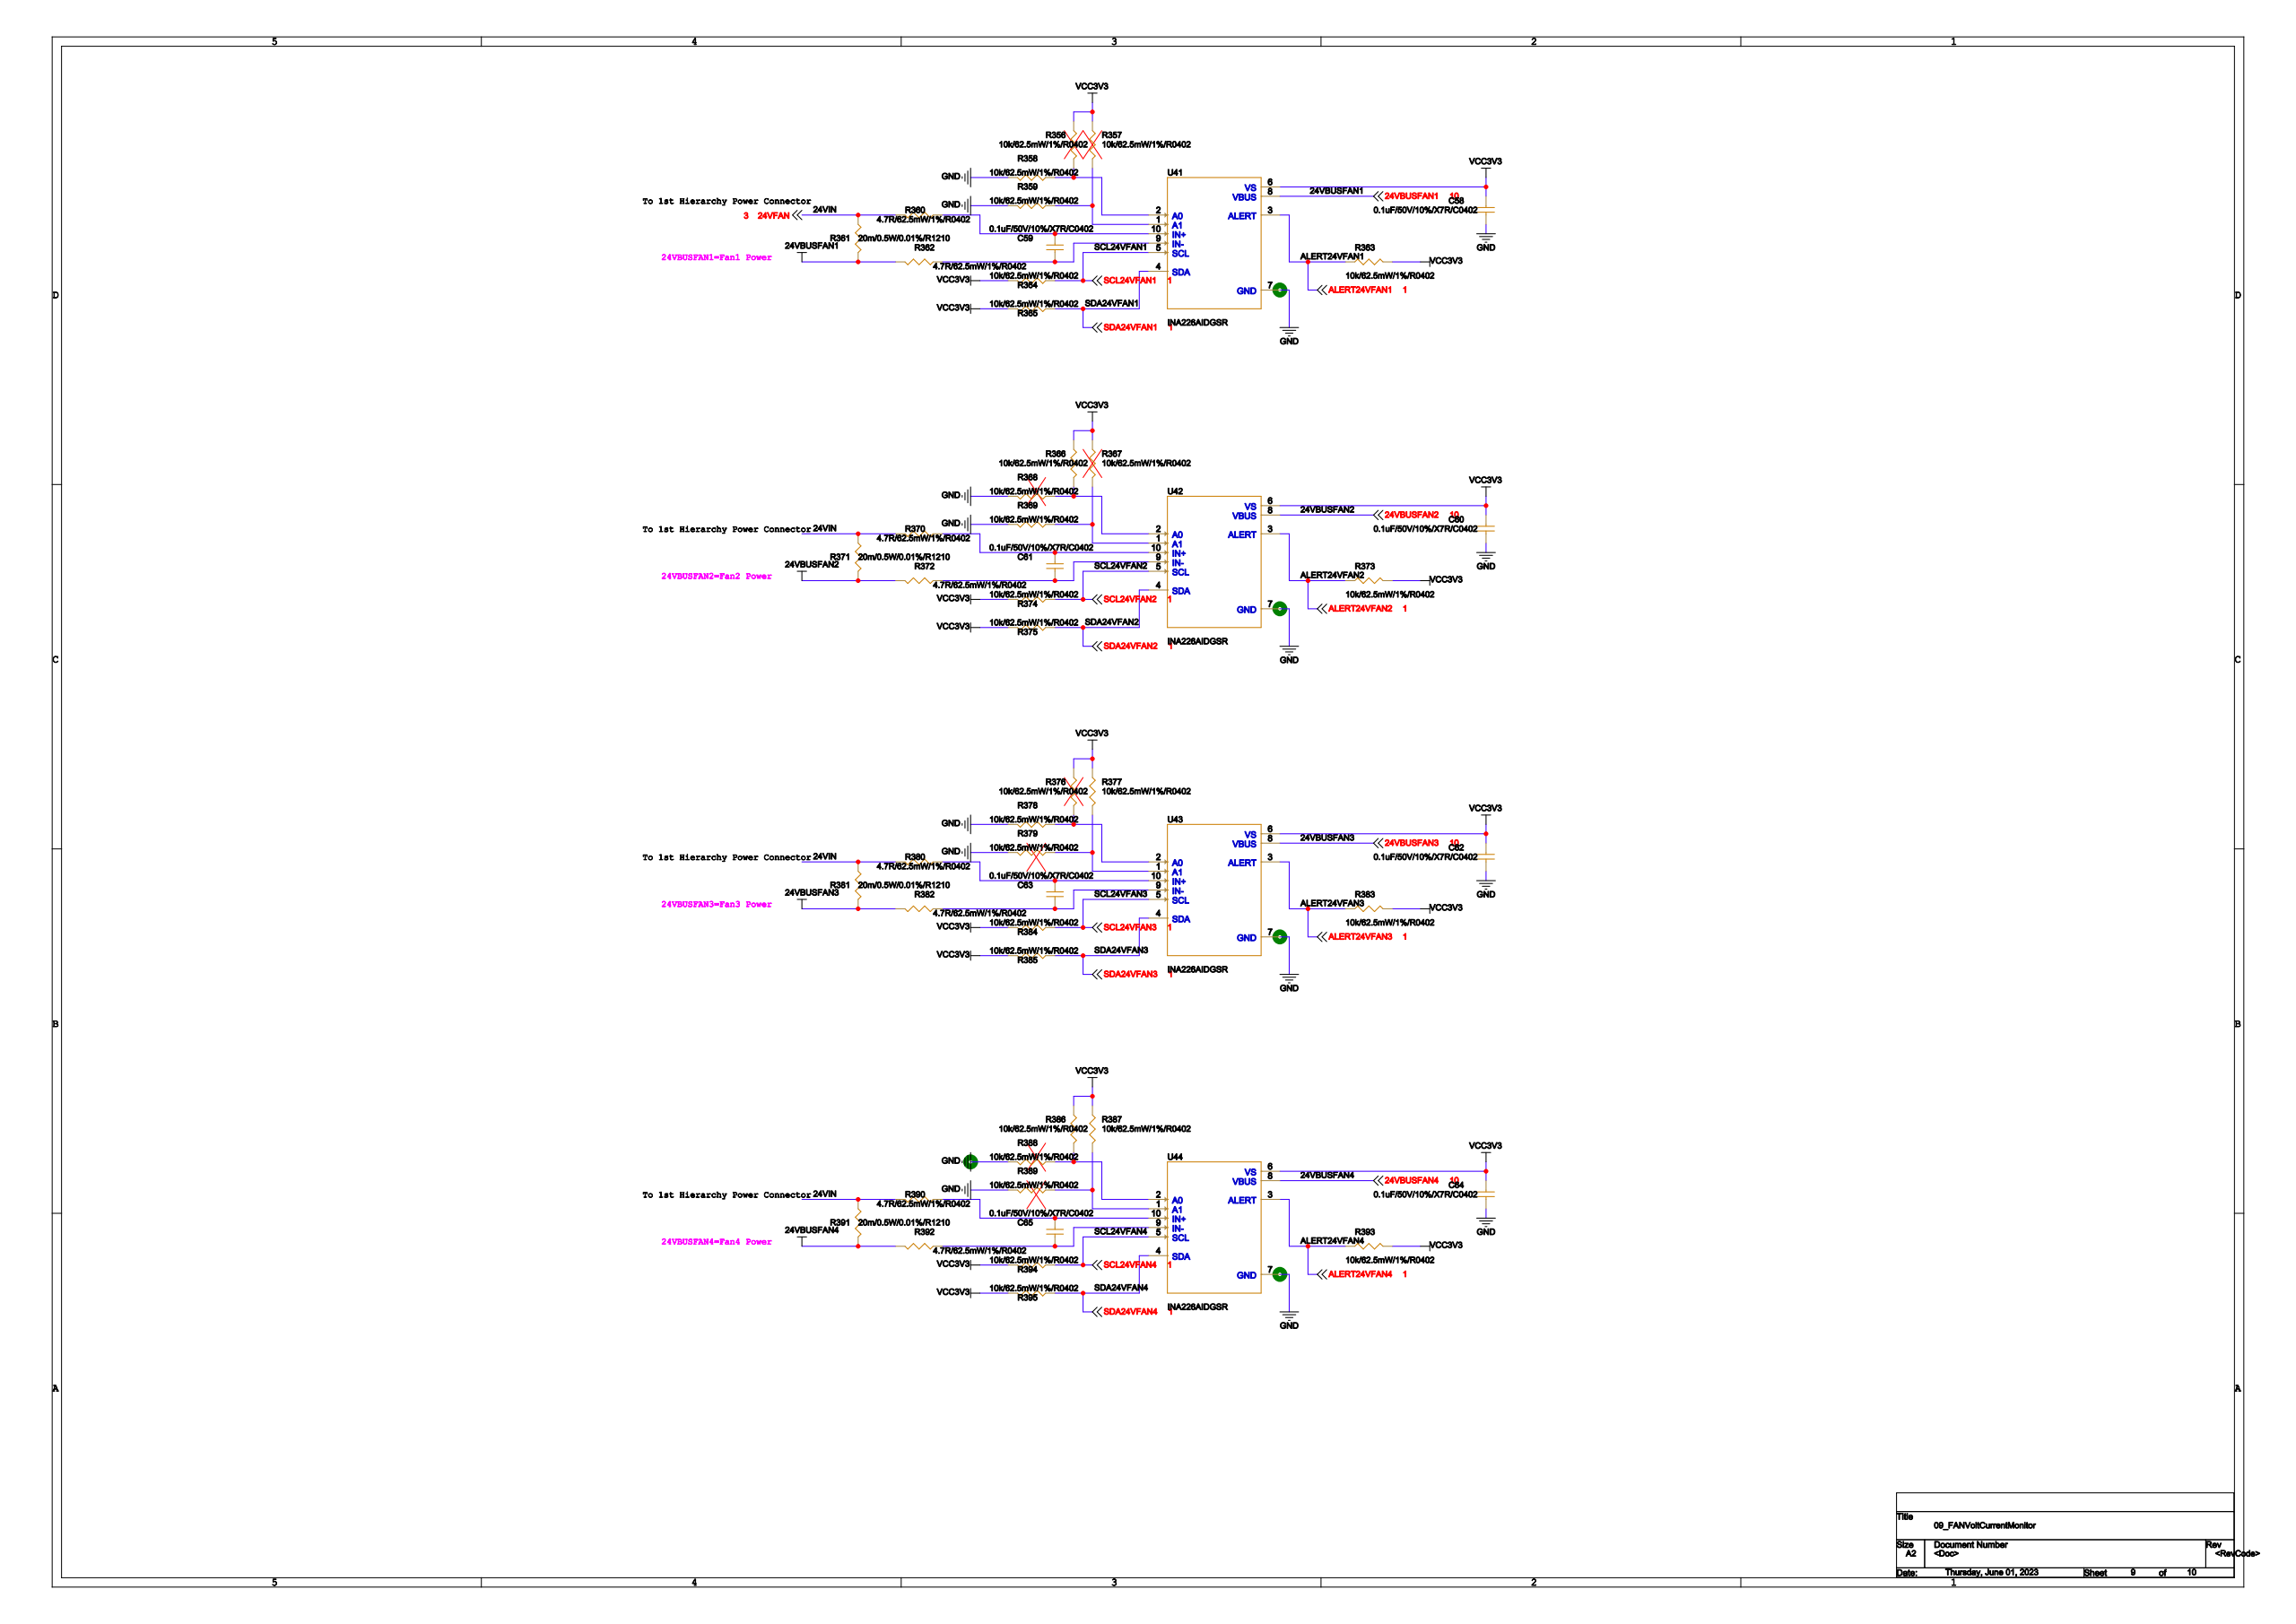Circuit board | Cadence Allegro | 480 parts | 625 nets | one sheet of the schematic
Parts on this sheet (reference | value | footprint):
C58 | 0.1uF/50V/10%/X7R/C0402 | 0402
C59 | 0.1uF/50V/10%/X7R/C0402 | 0402
C60 | 0.1uF/50V/10%/X7R/C0402 | 0402
C61 | 0.1uF/50V/10%/X7R/C0402 | 0402
C62 | 0.1uF/50V/10%/X7R/C0402 | 0402
C63 | 0.1uF/50V/10%/X7R/C0402 | 0402
C64 | 0.1uF/50V/10%/X7R/C0402 | 0402
C65 | 0.1uF/50V/10%/X7R/C0402 | 0402
R356 | 10k/62.5mW/1%/R0402 | 0402
R357 | 10k/62.5mW/1%/R0402 | 0402
R358 | 10k/62.5mW/1%/R0402 | 0402
R359 | 10k/62.5mW/1%/R0402 | 0402
R360 | 4.7R/62.5mW/1%/R0402 | 0402
R361 | 20m/0.5W/0.01%/R1210 | 1210
R362 | 4.7R/62.5mW/1%/R0402 | 0402
R363 | 10k/62.5mW/1%/R0402 | 0402
R364 | 10k/62.5mW/1%/R0402 | 0402
R365 | 10k/62.5mW/1%/R0402 | 0402
R366 | 10k/62.5mW/1%/R0402 | 0402
R367 | 10k/62.5mW/1%/R0402 | 0402
R368 | 10k/62.5mW/1%/R0402 | 0402
R369 | 10k/62.5mW/1%/R0402 | 0402
R370 | 4.7R/62.5mW/1%/R0402 | 0402
R371 | 20m/0.5W/0.01%/R1210 | 1210
R372 | 4.7R/62.5mW/1%/R0402 | 0402
R373 | 10k/62.5mW/1%/R0402 | 0402
R374 | 10k/62.5mW/1%/R0402 | 0402
R375 | 10k/62.5mW/1%/R0402 | 0402
R376 | 10k/62.5mW/1%/R0402 | 0402
R377 | 10k/62.5mW/1%/R0402 | 0402
R378 | 10k/62.5mW/1%/R0402 | 0402
R379 | 10k/62.5mW/1%/R0402 | 0402
R380 | 4.7R/62.5mW/1%/R0402 | 0402
R381 | 20m/0.5W/0.01%/R1210 | 1210
R382 | 4.7R/62.5mW/1%/R0402 | 0402
R383 | 10k/62.5mW/1%/R0402 | 0402
R384 | 10k/62.5mW/1%/R0402 | 0402
R385 | 10k/62.5mW/1%/R0402 | 0402
R386 | 10k/62.5mW/1%/R0402 | 0402
R387 | 10k/62.5mW/1%/R0402 | 0402
R388 | 10k/62.5mW/1%/R0402 | 0402
R389 | 10k/62.5mW/1%/R0402 | 0402
R390 | 4.7R/62.5mW/1%/R0402 | 0402
R391 | 20m/0.5W/0.01%/R1210 | 1210
R392 | 4.7R/62.5mW/1%/R0402 | 0402
R393 | 10k/62.5mW/1%/R0402 | 0402
R394 | 10k/62.5mW/1%/R0402 | 0402
R395 | 10k/62.5mW/1%/R0402 | 0402
U41 | INA226AIDGSR | SOP50P490X110-10N
U42 | INA226AIDGSR | SOP50P490X110-10N
U43 | INA226AIDGSR | SOP50P490X110-10N
U44 | INA226AIDGSR | SOP50P490X110-10N
Nets of these parts (net: part-pin ...):
AGND: C58-2 C60-2 C62-2 C64-2 R358-2 R359-2 R368-2 R369-2 R378-2 R379-2 R388-2 R389-2 U41-7 U42-7 U43-7 U44-7
BANK13_L5_N: R364-1 U41-5
ALERT24VFAN4: R393-1 U44-3
BANK13_L6_P: R365-1 U41-4
BANK13_L12_N: R395-1 U44-4
ALERT24VFAN1: R363-1 U41-3
BANK13_L4_N: R394-1 U44-5
BANK13_L5_P: R374-1 U42-5
ALERT24VFAN3: R383-1 U43-3
BANK13_L21_P: R375-1 U42-4
BANK13_L14_P: R385-1 U43-4
ALERT24VFAN2: R373-1 U42-3
BANK13_L17_N: R384-1 U43-5
3.3V: C58-1 C60-1 C62-1 C64-1 R356-1 R357-1 R363-2 R364-2 R365-2 R366-1 R367-1 R373-2 R374-2 R375-2 R376-1 R377-1 R383-2 R384-2 R385-2 R386-1 R387-1 R393-2 R394-2 R395-2 U41-6 U42-6 U43-6 U44-6
24VBUSFAN1: R361-2 R362-2 U41-8
24VBUSFAN4: R391-2 R392-2 U44-8
24VBUSFAN2: R371-2 R372-2 U42-8
24VBUSFAN3: R381-2 R382-2 U43-8
24VFAN: R360-2 R361-1 R370-2 R371-1 R380-2 R381-1 R390-2 R391-1
N23136700: C59-1 R360-1 U41-10
N23136726: C59-2 R362-1 U41-9
N23189446: C61-1 R370-1 U42-10
N23189612: C61-2 R372-1 U42-9
N23190079: C63-1 R380-1 U43-10
N23190245: C63-2 R382-1 U43-9
N23190745: C65-1 R390-1 U44-10
N23190911: C65-2 R392-1 U44-9
N23136475: R356-2 R358-1 U41-2
N23136485: R357-2 R359-1 U41-1
N23189541: R366-2 R368-1 U42-2
N23189547: R367-2 R369-1 U42-1
N23190174: R376-2 R378-1 U43-2
N23190180: R377-2 R379-1 U43-1
N23190840: R386-2 R388-1 U44-2
N23190846: R387-2 R389-1 U44-1